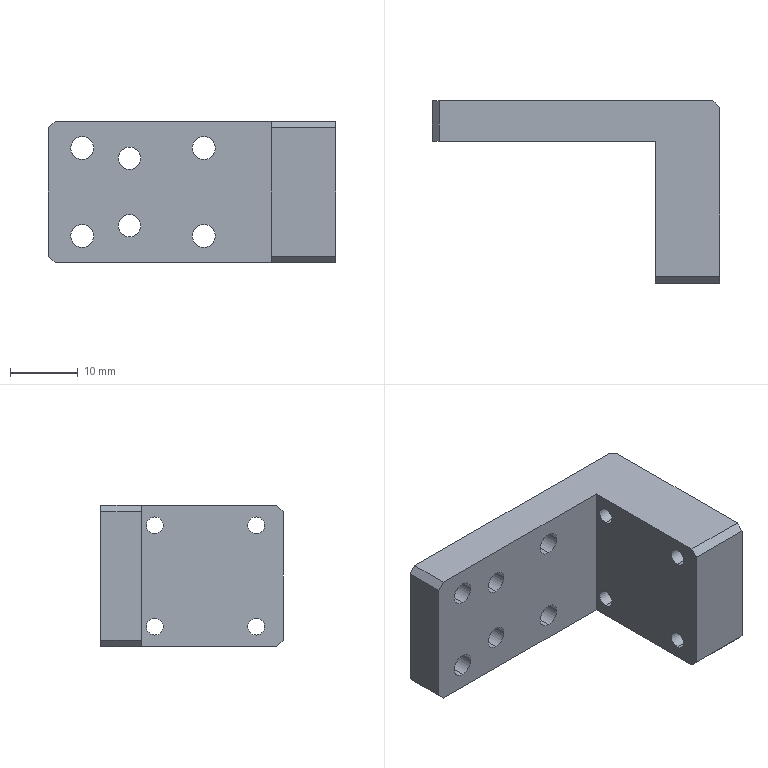Part | STEP file | FBDS-CS-002 | 1 solid | 45 faces | box 42.5 x 27 x 21 mm | volume 8750 mm3 | cylinder 28 | plane 17 | commonest cylinder face diameters 2.5 x8 3.4 x8 6 x8 3.3 x4
STEP:
#1=CARTESIAN_POINT('',(12.,-6.,3.85));
#2=VERTEX_POINT('',#1);
#3=CARTESIAN_POINT('',(12.,-6.,7.15));
#4=VERTEX_POINT('',#3);
#5=CARTESIAN_POINT('',(12.,-6.,5.5));
#6=DIRECTION('',(0.,1.,0.));
#7=DIRECTION('',(-1.,0.,0.));
#8=AXIS2_PLACEMENT_3D('',#5,#6,#7);
#9=CIRCLE('',#8,1.65);
#10=EDGE_CURVE('',#2,#4,#9,.T.);
#11=ORIENTED_EDGE('',*,*,#10,.F.);
#12=CARTESIAN_POINT('',(12.,0.,3.85));
#13=VERTEX_POINT('',#12);
#14=CARTESIAN_POINT('',(12.,0.,3.85));
#15=DIRECTION('',(0.,1.,0.));
#16=VECTOR('',#15,1000.);
#17=LINE('',#14,#16);
#18=EDGE_CURVE('',#2,#13,#17,.T.);
#19=ORIENTED_EDGE('',*,*,#18,.T.);
#20=CARTESIAN_POINT('',(12.,0.,7.15));
#21=VERTEX_POINT('',#20);
#22=CARTESIAN_POINT('',(12.,0.,5.5));
#23=DIRECTION('',(0.,1.,0.));
#24=DIRECTION('',(0.,0.,1.));
#25=AXIS2_PLACEMENT_3D('',#22,#23,#24);
#26=CIRCLE('',#25,1.65);
#27=EDGE_CURVE('',#13,#21,#26,.T.);
#28=ORIENTED_EDGE('',*,*,#27,.T.);
#29=CARTESIAN_POINT('',(12.,0.,7.15));
#30=DIRECTION('',(0.,1.,0.));
#31=VECTOR('',#30,1000.);
#32=LINE('',#29,#31);
#33=EDGE_CURVE('',#4,#21,#32,.T.);
#34=ORIENTED_EDGE('',*,*,#33,.F.);
#35=EDGE_LOOP('',(#11,#19,#28,#34));
#36=FACE_OUTER_BOUND('',#35,.T.);
#37=CARTESIAN_POINT('',(12.,0.,5.5));
#38=DIRECTION('',(0.,1.,0.));
#39=DIRECTION('',(0.,0.,1.));
#40=AXIS2_PLACEMENT_3D('',#37,#38,#39);
#41=CYLINDRICAL_SURFACE('',#40,1.65);
#42=ADVANCED_FACE('',(#36),#41,.F.);
#43=CARTESIAN_POINT('',(12.,-6.,13.85));
#44=VERTEX_POINT('',#43);
#45=CARTESIAN_POINT('',(12.,-6.,17.15));
#46=VERTEX_POINT('',#45);
#47=CARTESIAN_POINT('',(12.,-6.,15.5));
#48=DIRECTION('',(0.,1.,0.));
#49=DIRECTION('',(-1.,0.,0.));
#50=AXIS2_PLACEMENT_3D('',#47,#48,#49);
#51=CIRCLE('',#50,1.65);
#52=EDGE_CURVE('',#44,#46,#51,.T.);
#53=ORIENTED_EDGE('',*,*,#52,.F.);
#54=CARTESIAN_POINT('',(12.,0.,13.85));
#55=VERTEX_POINT('',#54);
#56=CARTESIAN_POINT('',(12.,0.,13.85));
#57=DIRECTION('',(0.,1.,0.));
#58=VECTOR('',#57,1000.);
#59=LINE('',#56,#58);
#60=EDGE_CURVE('',#44,#55,#59,.T.);
#61=ORIENTED_EDGE('',*,*,#60,.T.);
#62=CARTESIAN_POINT('',(12.,0.,17.15));
#63=VERTEX_POINT('',#62);
#64=CARTESIAN_POINT('',(12.,0.,15.5));
#65=DIRECTION('',(0.,1.,0.));
#66=DIRECTION('',(0.,0.,1.));
#67=AXIS2_PLACEMENT_3D('',#64,#65,#66);
#68=CIRCLE('',#67,1.65);
#69=EDGE_CURVE('',#55,#63,#68,.T.);
#70=ORIENTED_EDGE('',*,*,#69,.T.);
#71=CARTESIAN_POINT('',(12.,0.,17.15));
#72=DIRECTION('',(0.,1.,0.));
#73=VECTOR('',#72,1000.);
#74=LINE('',#71,#73);
#75=EDGE_CURVE('',#46,#63,#74,.T.);
#76=ORIENTED_EDGE('',*,*,#75,.F.);
#77=EDGE_LOOP('',(#53,#61,#70,#76));
#78=FACE_OUTER_BOUND('',#77,.T.);
#79=CARTESIAN_POINT('',(12.,0.,15.5));
#80=DIRECTION('',(0.,1.,0.));
#81=DIRECTION('',(0.,0.,1.));
#82=AXIS2_PLACEMENT_3D('',#79,#80,#81);
#83=CYLINDRICAL_SURFACE('',#82,1.65);
#84=ADVANCED_FACE('',(#78),#83,.F.);
#85=CARTESIAN_POINT('',(33.,-8.,4.25));
#86=VERTEX_POINT('',#85);
#87=CARTESIAN_POINT('',(33.,-8.,1.75));
#88=VERTEX_POINT('',#87);
#89=CARTESIAN_POINT('',(33.,-8.,3.));
#90=DIRECTION('',(1.,0.,0.));
#91=DIRECTION('',(0.,0.,-1.));
#92=AXIS2_PLACEMENT_3D('',#89,#90,#91);
#93=CIRCLE('',#92,1.25);
#94=EDGE_CURVE('',#86,#88,#93,.T.);
#95=ORIENTED_EDGE('',*,*,#94,.F.);
#96=CARTESIAN_POINT('',(42.5,-8.,4.25));
#97=VERTEX_POINT('',#96);
#98=CARTESIAN_POINT('',(42.5,-8.,4.25));
#99=DIRECTION('',(1.,0.,0.));
#100=VECTOR('',#99,1000.);
#101=LINE('',#98,#100);
#102=EDGE_CURVE('',#86,#97,#101,.T.);
#103=ORIENTED_EDGE('',*,*,#102,.T.);
#104=CARTESIAN_POINT('',(42.5,-8.,1.75));
#105=VERTEX_POINT('',#104);
#106=CARTESIAN_POINT('',(42.5,-8.,3.));
#107=DIRECTION('',(1.,0.,0.));
#108=DIRECTION('',(0.,0.,-1.));
#109=AXIS2_PLACEMENT_3D('',#106,#107,#108);
#110=CIRCLE('',#109,1.25);
#111=EDGE_CURVE('',#97,#105,#110,.T.);
#112=ORIENTED_EDGE('',*,*,#111,.T.);
#113=CARTESIAN_POINT('',(42.5,-8.,1.75));
#114=DIRECTION('',(1.,0.,0.));
#115=VECTOR('',#114,1000.);
#116=LINE('',#113,#115);
#117=EDGE_CURVE('',#88,#105,#116,.T.);
#118=ORIENTED_EDGE('',*,*,#117,.F.);
#119=EDGE_LOOP('',(#95,#103,#112,#118));
#120=FACE_OUTER_BOUND('',#119,.T.);
#121=CARTESIAN_POINT('',(42.5,-8.,3.));
#122=DIRECTION('',(1.,0.,0.));
#123=DIRECTION('',(0.,0.,-1.));
#124=AXIS2_PLACEMENT_3D('',#121,#122,#123);
#125=CYLINDRICAL_SURFACE('',#124,1.25);
#126=ADVANCED_FACE('',(#120),#125,.F.);
#127=CARTESIAN_POINT('',(33.,-8.,19.25));
#128=VERTEX_POINT('',#127);
#129=CARTESIAN_POINT('',(33.,-8.,16.75));
#130=VERTEX_POINT('',#129);
#131=CARTESIAN_POINT('',(33.,-8.,18.));
#132=DIRECTION('',(1.,0.,0.));
#133=DIRECTION('',(0.,0.,-1.));
#134=AXIS2_PLACEMENT_3D('',#131,#132,#133);
#135=CIRCLE('',#134,1.25);
#136=EDGE_CURVE('',#128,#130,#135,.T.);
#137=ORIENTED_EDGE('',*,*,#136,.F.);
#138=CARTESIAN_POINT('',(42.5,-8.,19.25));
#139=VERTEX_POINT('',#138);
#140=CARTESIAN_POINT('',(42.5,-8.,19.25));
#141=DIRECTION('',(1.,0.,0.));
#142=VECTOR('',#141,1000.);
#143=LINE('',#140,#142);
#144=EDGE_CURVE('',#128,#139,#143,.T.);
#145=ORIENTED_EDGE('',*,*,#144,.T.);
#146=CARTESIAN_POINT('',(42.5,-8.,16.75));
#147=VERTEX_POINT('',#146);
#148=CARTESIAN_POINT('',(42.5,-8.,18.));
#149=DIRECTION('',(1.,0.,0.));
#150=DIRECTION('',(0.,0.,-1.));
#151=AXIS2_PLACEMENT_3D('',#148,#149,#150);
#152=CIRCLE('',#151,1.25);
#153=EDGE_CURVE('',#139,#147,#152,.T.);
#154=ORIENTED_EDGE('',*,*,#153,.T.);
#155=CARTESIAN_POINT('',(42.5,-8.,16.75));
#156=DIRECTION('',(1.,0.,0.));
#157=VECTOR('',#156,1000.);
#158=LINE('',#155,#157);
#159=EDGE_CURVE('',#130,#147,#158,.T.);
#160=ORIENTED_EDGE('',*,*,#159,.F.);
#161=EDGE_LOOP('',(#137,#145,#154,#160));
#162=FACE_OUTER_BOUND('',#161,.T.);
#163=CARTESIAN_POINT('',(42.5,-8.,18.));
#164=DIRECTION('',(1.,0.,0.));
#165=DIRECTION('',(0.,0.,-1.));
#166=AXIS2_PLACEMENT_3D('',#163,#164,#165);
#167=CYLINDRICAL_SURFACE('',#166,1.25);
#168=ADVANCED_FACE('',(#162),#167,.F.);
#169=CARTESIAN_POINT('',(33.,-23.,4.25));
#170=VERTEX_POINT('',#169);
#171=CARTESIAN_POINT('',(33.,-23.,1.75));
#172=VERTEX_POINT('',#171);
#173=CARTESIAN_POINT('',(33.,-23.,3.));
#174=DIRECTION('',(1.,0.,0.));
#175=DIRECTION('',(0.,0.,-1.));
#176=AXIS2_PLACEMENT_3D('',#173,#174,#175);
#177=CIRCLE('',#176,1.25);
#178=EDGE_CURVE('',#170,#172,#177,.T.);
#179=ORIENTED_EDGE('',*,*,#178,.F.);
#180=CARTESIAN_POINT('',(42.5,-23.,4.25));
#181=VERTEX_POINT('',#180);
#182=CARTESIAN_POINT('',(42.5,-23.,4.25));
#183=DIRECTION('',(1.,0.,0.));
#184=VECTOR('',#183,1000.);
#185=LINE('',#182,#184);
#186=EDGE_CURVE('',#170,#181,#185,.T.);
#187=ORIENTED_EDGE('',*,*,#186,.T.);
#188=CARTESIAN_POINT('',(42.5,-23.,1.75));
#189=VERTEX_POINT('',#188);
#190=CARTESIAN_POINT('',(42.5,-23.,3.));
#191=DIRECTION('',(1.,0.,0.));
#192=DIRECTION('',(0.,0.,-1.));
#193=AXIS2_PLACEMENT_3D('',#190,#191,#192);
#194=CIRCLE('',#193,1.25);
#195=EDGE_CURVE('',#181,#189,#194,.T.);
#196=ORIENTED_EDGE('',*,*,#195,.T.);
#197=CARTESIAN_POINT('',(42.5,-23.,1.75));
#198=DIRECTION('',(1.,0.,0.));
#199=VECTOR('',#198,1000.);
#200=LINE('',#197,#199);
#201=EDGE_CURVE('',#172,#189,#200,.T.);
#202=ORIENTED_EDGE('',*,*,#201,.F.);
#203=EDGE_LOOP('',(#179,#187,#196,#202));
#204=FACE_OUTER_BOUND('',#203,.T.);
#205=CARTESIAN_POINT('',(42.5,-23.,3.));
#206=DIRECTION('',(1.,0.,0.));
#207=DIRECTION('',(0.,0.,-1.));
#208=AXIS2_PLACEMENT_3D('',#205,#206,#207);
#209=CYLINDRICAL_SURFACE('',#208,1.25);
#210=ADVANCED_FACE('',(#204),#209,.F.);
#211=CARTESIAN_POINT('',(33.,-23.,19.25));
#212=VERTEX_POINT('',#211);
#213=CARTESIAN_POINT('',(33.,-23.,16.75));
#214=VERTEX_POINT('',#213);
#215=CARTESIAN_POINT('',(33.,-23.,18.));
#216=DIRECTION('',(1.,0.,0.));
#217=DIRECTION('',(0.,0.,-1.));
#218=AXIS2_PLACEMENT_3D('',#215,#216,#217);
#219=CIRCLE('',#218,1.25);
#220=EDGE_CURVE('',#212,#214,#219,.T.);
#221=ORIENTED_EDGE('',*,*,#220,.F.);
#222=CARTESIAN_POINT('',(42.5,-23.,19.25));
#223=VERTEX_POINT('',#222);
#224=CARTESIAN_POINT('',(42.5,-23.,19.25));
#225=DIRECTION('',(1.,0.,0.));
#226=VECTOR('',#225,1000.);
#227=LINE('',#224,#226);
#228=EDGE_CURVE('',#212,#223,#227,.T.);
#229=ORIENTED_EDGE('',*,*,#228,.T.);
#230=CARTESIAN_POINT('',(42.5,-23.,16.75));
#231=VERTEX_POINT('',#230);
#232=CARTESIAN_POINT('',(42.5,-23.,18.));
#233=DIRECTION('',(1.,0.,0.));
#234=DIRECTION('',(0.,0.,-1.));
#235=AXIS2_PLACEMENT_3D('',#232,#233,#234);
#236=CIRCLE('',#235,1.25);
#237=EDGE_CURVE('',#223,#231,#236,.T.);
#238=ORIENTED_EDGE('',*,*,#237,.T.);
#239=CARTESIAN_POINT('',(42.5,-23.,16.75));
#240=DIRECTION('',(1.,0.,0.));
#241=VECTOR('',#240,1000.);
#242=LINE('',#239,#241);
#243=EDGE_CURVE('',#214,#231,#242,.T.);
#244=ORIENTED_EDGE('',*,*,#243,.F.);
#245=EDGE_LOOP('',(#221,#229,#238,#244));
#246=FACE_OUTER_BOUND('',#245,.T.);
#247=CARTESIAN_POINT('',(42.5,-23.,18.));
#248=DIRECTION('',(1.,0.,0.));
#249=DIRECTION('',(0.,0.,-1.));
#250=AXIS2_PLACEMENT_3D('',#247,#248,#249);
#251=CYLINDRICAL_SURFACE('',#250,1.25);
#252=ADVANCED_FACE('',(#246),#251,.F.);
#253=CARTESIAN_POINT('',(5.,-3.4,1.));
#254=VERTEX_POINT('',#253);
#255=CARTESIAN_POINT('',(5.,-3.4,7.));
#256=VERTEX_POINT('',#255);
#257=CARTESIAN_POINT('',(5.,-3.4,4.));
#258=DIRECTION('',(0.,1.,0.));
#259=DIRECTION('',(0.,0.,1.));
#260=AXIS2_PLACEMENT_3D('',#257,#258,#259);
#261=CIRCLE('',#260,3.);
#262=EDGE_CURVE('',#254,#256,#261,.T.);
#263=ORIENTED_EDGE('',*,*,#262,.F.);
#264=CARTESIAN_POINT('',(5.,0.,1.));
#265=VERTEX_POINT('',#264);
#266=CARTESIAN_POINT('',(5.,0.,1.));
#267=DIRECTION('',(0.,1.,0.));
#268=VECTOR('',#267,1000.);
#269=LINE('',#266,#268);
#270=EDGE_CURVE('',#254,#265,#269,.T.);
#271=ORIENTED_EDGE('',*,*,#270,.T.);
#272=CARTESIAN_POINT('',(5.,0.,7.));
#273=VERTEX_POINT('',#272);
#274=CARTESIAN_POINT('',(5.,0.,4.));
#275=DIRECTION('',(0.,1.,0.));
#276=DIRECTION('',(0.,0.,1.));
#277=AXIS2_PLACEMENT_3D('',#274,#275,#276);
#278=CIRCLE('',#277,3.);
#279=EDGE_CURVE('',#265,#273,#278,.T.);
#280=ORIENTED_EDGE('',*,*,#279,.T.);
#281=CARTESIAN_POINT('',(5.,0.,7.));
#282=DIRECTION('',(0.,1.,0.));
#283=VECTOR('',#282,1000.);
#284=LINE('',#281,#283);
#285=EDGE_CURVE('',#256,#273,#284,.T.);
#286=ORIENTED_EDGE('',*,*,#285,.F.);
#287=EDGE_LOOP('',(#263,#271,#280,#286));
#288=FACE_OUTER_BOUND('',#287,.T.);
#289=CARTESIAN_POINT('',(5.,0.,4.));
#290=DIRECTION('',(0.,1.,0.));
#291=DIRECTION('',(0.,0.,1.));
#292=AXIS2_PLACEMENT_3D('',#289,#290,#291);
#293=CYLINDRICAL_SURFACE('',#292,3.);
#294=ADVANCED_FACE('',(#288),#293,.F.);
#295=CARTESIAN_POINT('',(5.,-6.,2.3));
#296=VERTEX_POINT('',#295);
#297=CARTESIAN_POINT('',(5.,-6.,5.7));
#298=VERTEX_POINT('',#297);
#299=CARTESIAN_POINT('',(5.,-6.,4.));
#300=DIRECTION('',(0.,1.,0.));
#301=DIRECTION('',(-1.,0.,0.));
#302=AXIS2_PLACEMENT_3D('',#299,#300,#301);
#303=CIRCLE('',#302,1.7);
#304=EDGE_CURVE('',#296,#298,#303,.T.);
#305=ORIENTED_EDGE('',*,*,#304,.F.);
#306=CARTESIAN_POINT('',(5.,-3.4,2.3));
#307=VERTEX_POINT('',#306);
#308=CARTESIAN_POINT('',(5.,0.,2.3));
#309=DIRECTION('',(0.,1.,0.));
#310=VECTOR('',#309,1000.);
#311=LINE('',#308,#310);
#312=EDGE_CURVE('',#296,#307,#311,.T.);
#313=ORIENTED_EDGE('',*,*,#312,.T.);
#314=CARTESIAN_POINT('',(5.,-3.4,5.7));
#315=VERTEX_POINT('',#314);
#316=CARTESIAN_POINT('',(5.,-3.4,4.));
#317=DIRECTION('',(0.,1.,0.));
#318=DIRECTION('',(0.,0.,1.));
#319=AXIS2_PLACEMENT_3D('',#316,#317,#318);
#320=CIRCLE('',#319,1.7);
#321=EDGE_CURVE('',#307,#315,#320,.T.);
#322=ORIENTED_EDGE('',*,*,#321,.T.);
#323=CARTESIAN_POINT('',(5.,0.,5.7));
#324=DIRECTION('',(0.,1.,0.));
#325=VECTOR('',#324,1000.);
#326=LINE('',#323,#325);
#327=EDGE_CURVE('',#298,#315,#326,.T.);
#328=ORIENTED_EDGE('',*,*,#327,.F.);
#329=EDGE_LOOP('',(#305,#313,#322,#328));
#330=FACE_OUTER_BOUND('',#329,.T.);
#331=CARTESIAN_POINT('',(5.,0.,4.));
#332=DIRECTION('',(0.,1.,0.));
#333=DIRECTION('',(0.,0.,1.));
#334=AXIS2_PLACEMENT_3D('',#331,#332,#333);
#335=CYLINDRICAL_SURFACE('',#334,1.7);
#336=ADVANCED_FACE('',(#330),#335,.F.);
#337=CARTESIAN_POINT('',(23.,-3.4,1.));
#338=VERTEX_POINT('',#337);
#339=CARTESIAN_POINT('',(23.,-3.4,7.));
#340=VERTEX_POINT('',#339);
#341=CARTESIAN_POINT('',(23.,-3.4,4.));
#342=DIRECTION('',(0.,1.,0.));
#343=DIRECTION('',(0.,0.,1.));
#344=AXIS2_PLACEMENT_3D('',#341,#342,#343);
#345=CIRCLE('',#344,3.);
#346=EDGE_CURVE('',#338,#340,#345,.T.);
#347=ORIENTED_EDGE('',*,*,#346,.F.);
#348=CARTESIAN_POINT('',(23.,0.,1.));
#349=VERTEX_POINT('',#348);
#350=CARTESIAN_POINT('',(23.,0.,1.));
#351=DIRECTION('',(0.,1.,0.));
#352=VECTOR('',#351,1000.);
#353=LINE('',#350,#352);
#354=EDGE_CURVE('',#338,#349,#353,.T.);
#355=ORIENTED_EDGE('',*,*,#354,.T.);
#356=CARTESIAN_POINT('',(23.,0.,7.));
#357=VERTEX_POINT('',#356);
#358=CARTESIAN_POINT('',(23.,0.,4.));
#359=DIRECTION('',(0.,1.,0.));
#360=DIRECTION('',(0.,0.,1.));
#361=AXIS2_PLACEMENT_3D('',#358,#359,#360);
#362=CIRCLE('',#361,3.);
#363=EDGE_CURVE('',#349,#357,#362,.T.);
#364=ORIENTED_EDGE('',*,*,#363,.T.);
#365=CARTESIAN_POINT('',(23.,0.,7.));
#366=DIRECTION('',(0.,1.,0.));
#367=VECTOR('',#366,1000.);
#368=LINE('',#365,#367);
#369=EDGE_CURVE('',#340,#357,#368,.T.);
#370=ORIENTED_EDGE('',*,*,#369,.F.);
#371=EDGE_LOOP('',(#347,#355,#364,#370));
#372=FACE_OUTER_BOUND('',#371,.T.);
#373=CARTESIAN_POINT('',(23.,0.,4.));
#374=DIRECTION('',(0.,1.,0.));
#375=DIRECTION('',(0.,0.,1.));
#376=AXIS2_PLACEMENT_3D('',#373,#374,#375);
#377=CYLINDRICAL_SURFACE('',#376,3.);
#378=ADVANCED_FACE('',(#372),#377,.F.);
#379=CARTESIAN_POINT('',(23.,-6.,2.3));
#380=VERTEX_POINT('',#379);
#381=CARTESIAN_POINT('',(23.,-6.,5.7));
#382=VERTEX_POINT('',#381);
#383=CARTESIAN_POINT('',(23.,-6.,4.));
#384=DIRECTION('',(0.,1.,0.));
#385=DIRECTION('',(-1.,0.,0.));
#386=AXIS2_PLACEMENT_3D('',#383,#384,#385);
#387=CIRCLE('',#386,1.7);
#388=EDGE_CURVE('',#380,#382,#387,.T.);
#389=ORIENTED_EDGE('',*,*,#388,.F.);
#390=CARTESIAN_POINT('',(23.,-3.4,2.3));
#391=VERTEX_POINT('',#390);
#392=CARTESIAN_POINT('',(23.,0.,2.3));
#393=DIRECTION('',(0.,1.,0.));
#394=VECTOR('',#393,1000.);
#395=LINE('',#392,#394);
#396=EDGE_CURVE('',#380,#391,#395,.T.);
#397=ORIENTED_EDGE('',*,*,#396,.T.);
#398=CARTESIAN_POINT('',(23.,-3.4,5.7));
#399=VERTEX_POINT('',#398);
#400=CARTESIAN_POINT('',(23.,-3.4,4.));
#401=DIRECTION('',(0.,1.,0.));
#402=DIRECTION('',(0.,0.,1.));
#403=AXIS2_PLACEMENT_3D('',#400,#401,#402);
#404=CIRCLE('',#403,1.7);
#405=EDGE_CURVE('',#391,#399,#404,.T.);
#406=ORIENTED_EDGE('',*,*,#405,.T.);
#407=CARTESIAN_POINT('',(23.,0.,5.7));
#408=DIRECTION('',(0.,1.,0.));
#409=VECTOR('',#408,1000.);
#410=LINE('',#407,#409);
#411=EDGE_CURVE('',#382,#399,#410,.T.);
#412=ORIENTED_EDGE('',*,*,#411,.F.);
#413=EDGE_LOOP('',(#389,#397,#406,#412));
#414=FACE_OUTER_BOUND('',#413,.T.);
#415=CARTESIAN_POINT('',(23.,0.,4.));
#416=DIRECTION('',(0.,1.,0.));
#417=DIRECTION('',(0.,0.,1.));
#418=AXIS2_PLACEMENT_3D('',#415,#416,#417);
#419=CYLINDRICAL_SURFACE('',#418,1.7);
#420=ADVANCED_FACE('',(#414),#419,.F.);
#421=CARTESIAN_POINT('',(23.,-3.4,14.));
#422=VERTEX_POINT('',#421);
#423=CARTESIAN_POINT('',(23.,-3.4,20.));
#424=VERTEX_POINT('',#423);
#425=CARTESIAN_POINT('',(23.,-3.4,17.));
#426=DIRECTION('',(0.,1.,0.));
#427=DIRECTION('',(0.,0.,1.));
#428=AXIS2_PLACEMENT_3D('',#425,#426,#427);
#429=CIRCLE('',#428,3.);
#430=EDGE_CURVE('',#422,#424,#429,.T.);
#431=ORIENTED_EDGE('',*,*,#430,.F.);
#432=CARTESIAN_POINT('',(23.,0.,14.));
#433=VERTEX_POINT('',#432);
#434=CARTESIAN_POINT('',(23.,0.,14.));
#435=DIRECTION('',(0.,1.,0.));
#436=VECTOR('',#435,1000.);
#437=LINE('',#434,#436);
#438=EDGE_CURVE('',#422,#433,#437,.T.);
#439=ORIENTED_EDGE('',*,*,#438,.T.);
#440=CARTESIAN_POINT('',(23.,0.,20.));
#441=VERTEX_POINT('',#440);
#442=CARTESIAN_POINT('',(23.,0.,17.));
#443=DIRECTION('',(0.,1.,0.));
#444=DIRECTION('',(0.,0.,1.));
#445=AXIS2_PLACEMENT_3D('',#442,#443,#444);
#446=CIRCLE('',#445,3.);
#447=EDGE_CURVE('',#433,#441,#446,.T.);
#448=ORIENTED_EDGE('',*,*,#447,.T.);
#449=CARTESIAN_POINT('',(23.,0.,20.));
#450=DIRECTION('',(0.,1.,0.));
#451=VECTOR('',#450,1000.);
#452=LINE('',#449,#451);
#453=EDGE_CURVE('',#424,#441,#452,.T.);
#454=ORIENTED_EDGE('',*,*,#453,.F.);
#455=EDGE_LOOP('',(#431,#439,#448,#454));
#456=FACE_OUTER_BOUND('',#455,.T.);
#457=CARTESIAN_POINT('',(23.,0.,17.));
#458=DIRECTION('',(0.,1.,0.));
#459=DIRECTION('',(0.,0.,1.));
#460=AXIS2_PLACEMENT_3D('',#457,#458,#459);
#461=CYLINDRICAL_SURFACE('',#460,3.);
#462=ADVANCED_FACE('',(#456),#461,.F.);
#463=CARTESIAN_POINT('',(23.,-6.,15.3));
#464=VERTEX_POINT('',#463);
#465=CARTESIAN_POINT('',(23.,-6.,18.7));
#466=VERTEX_POINT('',#465);
#467=CARTESIAN_POINT('',(23.,-6.,17.));
#468=DIRECTION('',(0.,1.,0.));
#469=DIRECTION('',(-1.,0.,0.));
#470=AXIS2_PLACEMENT_3D('',#467,#468,#469);
#471=CIRCLE('',#470,1.7);
#472=EDGE_CURVE('',#464,#466,#471,.T.);
#473=ORIENTED_EDGE('',*,*,#472,.F.);
#474=CARTESIAN_POINT('',(23.,-3.4,15.3));
#475=VERTEX_POINT('',#474);
#476=CARTESIAN_POINT('',(23.,0.,15.3));
#477=DIRECTION('',(0.,1.,0.));
#478=VECTOR('',#477,1000.);
#479=LINE('',#476,#478);
#480=EDGE_CURVE('',#464,#475,#479,.T.);
#481=ORIENTED_EDGE('',*,*,#480,.T.);
#482=CARTESIAN_POINT('',(23.,-3.4,18.7));
#483=VERTEX_POINT('',#482);
#484=CARTESIAN_POINT('',(23.,-3.4,17.));
#485=DIRECTION('',(0.,1.,0.));
#486=DIRECTION('',(0.,0.,1.));
#487=AXIS2_PLACEMENT_3D('',#484,#485,#486);
#488=CIRCLE('',#487,1.7);
#489=EDGE_CURVE('',#475,#483,#488,.T.);
#490=ORIENTED_EDGE('',*,*,#489,.T.);
#491=CARTESIAN_POINT('',(23.,0.,18.7));
#492=DIRECTION('',(0.,1.,0.));
#493=VECTOR('',#492,1000.);
#494=LINE('',#491,#493);
#495=EDGE_CURVE('',#466,#483,#494,.T.);
#496=ORIENTED_EDGE('',*,*,#495,.F.);
#497=EDGE_LOOP('',(#473,#481,#490,#496));
#498=FACE_OUTER_BOUND('',#497,.T.);
#499=CARTESIAN_POINT('',(23.,0.,17.));
#500=DIRECTION('',(0.,1.,0.));
#501=DIRECTION('',(0.,0.,1.));
#502=AXIS2_PLACEMENT_3D('',#499,#500,#501);
#503=CYLINDRICAL_SURFACE('',#502,1.7);
#504=ADVANCED_FACE('',(#498),#503,.F.);
#505=CARTESIAN_POINT('',(5.,-3.4,14.));
#506=VERTEX_POINT('',#505);
#507=CARTESIAN_POINT('',(5.,-3.4,20.));
#508=VERTEX_POINT('',#507);
#509=CARTESIAN_POINT('',(5.,-3.4,17.));
#510=DIRECTION('',(0.,1.,0.));
#511=DIRECTION('',(0.,0.,1.));
#512=AXIS2_PLACEMENT_3D('',#509,#510,#511);
#513=CIRCLE('',#512,3.);
#514=EDGE_CURVE('',#506,#508,#513,.T.);
#515=ORIENTED_EDGE('',*,*,#514,.F.);
#516=CARTESIAN_POINT('',(5.,0.,14.));
#517=VERTEX_POINT('',#516);
#518=CARTESIAN_POINT('',(5.,0.,14.));
#519=DIRECTION('',(0.,1.,0.));
#520=VECTOR('',#519,1000.);
#521=LINE('',#518,#520);
#522=EDGE_CURVE('',#506,#517,#521,.T.);
#523=ORIENTED_EDGE('',*,*,#522,.T.);
#524=CARTESIAN_POINT('',(5.,0.,20.));
#525=VERTEX_POINT('',#524);
#526=CARTESIAN_POINT('',(5.,0.,17.));
#527=DIRECTION('',(0.,1.,0.));
#528=DIRECTION('',(0.,0.,1.));
#529=AXIS2_PLACEMENT_3D('',#526,#527,#528);
#530=CIRCLE('',#529,3.);
#531=EDGE_CURVE('',#517,#525,#530,.T.);
#532=ORIENTED_EDGE('',*,*,#531,.T.);
#533=CARTESIAN_POINT('',(5.,0.,20.));
#534=DIRECTION('',(0.,1.,0.));
#535=VECTOR('',#534,1000.);
#536=LINE('',#533,#535);
#537=EDGE_CURVE('',#508,#525,#536,.T.);
#538=ORIENTED_EDGE('',*,*,#537,.F.);
#539=EDGE_LOOP('',(#515,#523,#532,#538));
#540=FACE_OUTER_BOUND('',#539,.T.);
#541=CARTESIAN_POINT('',(5.,0.,17.));
#542=DIRECTION('',(0.,1.,0.));
#543=DIRECTION('',(0.,0.,1.));
#544=AXIS2_PLACEMENT_3D('',#541,#542,#543);
#545=CYLINDRICAL_SURFACE('',#544,3.);
#546=ADVANCED_FACE('',(#540),#545,.F.);
#547=CARTESIAN_POINT('',(5.,-6.,15.3));
#548=VERTEX_POINT('',#547);
#549=CARTESIAN_POINT('',(5.,-6.,18.7));
#550=VERTEX_POINT('',#549);
#551=CARTESIAN_POINT('',(5.,-6.,17.));
#552=DIRECTION('',(0.,1.,0.));
#553=DIRECTION('',(-1.,0.,0.));
#554=AXIS2_PLACEMENT_3D('',#551,#552,#553);
#555=CIRCLE('',#554,1.7);
#556=EDGE_CURVE('',#548,#550,#555,.T.);
#557=ORIENTED_EDGE('',*,*,#556,.F.);
#558=CARTESIAN_POINT('',(5.,-3.4,15.3));
#559=VERTEX_POINT('',#558);
#560=CARTESIAN_POINT('',(5.,0.,15.3));
#561=DIRECTION('',(0.,1.,0.));
#562=VECTOR('',#561,1000.);
#563=LINE('',#560,#562);
#564=EDGE_CURVE('',#548,#559,#563,.T.);
#565=ORIENTED_EDGE('',*,*,#564,.T.);
#566=CARTESIAN_POINT('',(5.,-3.4,18.7));
#567=VERTEX_POINT('',#566);
#568=CARTESIAN_POINT('',(5.,-3.4,17.));
#569=DIRECTION('',(0.,1.,0.));
#570=DIRECTION('',(0.,0.,1.));
#571=AXIS2_PLACEMENT_3D('',#568,#569,#570);
#572=CIRCLE('',#571,1.7);
#573=EDGE_CURVE('',#559,#567,#572,.T.);
#574=ORIENTED_EDGE('',*,*,#573,.T.);
#575=CARTESIAN_POINT('',(5.,0.,18.7));
#576=DIRECTION('',(0.,1.,0.));
#577=VECTOR('',#576,1000.);
#578=LINE('',#575,#577);
#579=EDGE_CURVE('',#550,#567,#578,.T.);
#580=ORIENTED_EDGE('',*,*,#579,.F.);
#581=EDGE_LOOP('',(#557,#565,#574,#580));
#582=FACE_OUTER_BOUND('',#581,.T.);
#583=CARTESIAN_POINT('',(5.,0.,17.));
#584=DIRECTION('',(0.,1.,0.));
#585=DIRECTION('',(0.,0.,1.));
#586=AXIS2_PLACEMENT_3D('',#583,#584,#585);
#587=CYLINDRICAL_SURFACE('',#586,1.7);
#588=ADVANCED_FACE('',(#582),#587,.F.);
#589=CARTESIAN_POINT('',(0.,-6.,20.));
#590=VERTEX_POINT('',#589);
#591=CARTESIAN_POINT('',(0.,-6.,1.));
#592=VERTEX_POINT('',#591);
#593=CARTESIAN_POINT('',(0.,-6.,21.));
#594=DIRECTION('',(0.,0.,-1.));
#595=VECTOR('',#594,1000.);
#596=LINE('',#593,#595);
#597=EDGE_CURVE('',#590,#592,#596,.T.);
#598=ORIENTED_EDGE('',*,*,#597,.F.);
#599=CARTESIAN_POINT('',(0.,0.,20.));
#600=VERTEX_POINT('',#599);
#601=CARTESIAN_POINT('',(0.,-6.,20.));
#602=DIRECTION('',(0.,1.,0.));
#603=VECTOR('',#602,1000.);
#604=LINE('',#601,#603);
#605=EDGE_CURVE('',#590,#600,#604,.T.);
#606=ORIENTED_EDGE('',*,*,#605,.T.);
#607=CARTESIAN_POINT('',(0.,0.,1.));
#608=VERTEX_POINT('',#607);
#609=CARTESIAN_POINT('',(0.,0.,21.));
#610=DIRECTION('',(0.,0.,-1.));
#611=VECTOR('',#610,1000.);
#612=LINE('',#609,#611);
#613=EDGE_CURVE('',#600,#608,#612,.T.);
#614=ORIENTED_EDGE('',*,*,#613,.T.);
#615=CARTESIAN_POINT('',(0.,-6.,1.));
#616=DIRECTION('',(0.,-1.,0.));
#617=VECTOR('',#616,1000.);
#618=LINE('',#615,#617);
#619=EDGE_CURVE('',#608,#592,#618,.T.);
#620=ORIENTED_EDGE('',*,*,#619,.T.);
#621=EDGE_LOOP('',(#598,#606,#614,#620));
#622=FACE_OUTER_BOUND('',#621,.T.);
#623=CARTESIAN_POINT('',(0.,-6.,21.));
#624=DIRECTION('',(1.,0.,0.));
#625=DIRECTION('',(0.,0.,-1.));
#626=AXIS2_PLACEMENT_3D('',#623,#624,#625);
#627=PLANE('',#626);
#628=ADVANCED_FACE('',(#622),#627,.F.);
#629=CARTESIAN_POINT('',(12.,-6.,5.5));
#630=DIRECTION('',(0.,1.,0.));
#631=DIRECTION('',(-1.,0.,0.));
#632=AXIS2_PLACEMENT_3D('',#629,#630,#631);
#633=CIRCLE('',#632,1.65);
#634=EDGE_CURVE('',#4,#2,#633,.T.);
#635=ORIENTED_EDGE('',*,*,#634,.T.);
#636=ORIENTED_EDGE('',*,*,#10,.T.);
#637=EDGE_LOOP('',(#635,#636));
#638=FACE_BOUND('',#637,.T.);
#639=CARTESIAN_POINT('',(12.,-6.,15.5));
#640=DIRECTION('',(0.,1.,0.));
#641=DIRECTION('',(-1.,0.,0.));
#642=AXIS2_PLACEMENT_3D('',#639,#640,#641);
#643=CIRCLE('',#642,1.65);
#644=EDGE_CURVE('',#46,#44,#643,.T.);
#645=ORIENTED_EDGE('',*,*,#644,.T.);
#646=ORIENTED_EDGE('',*,*,#52,.T.);
#647=EDGE_LOOP('',(#645,#646));
#648=FACE_BOUND('',#647,.T.);
#649=CARTESIAN_POINT('',(5.,-6.,4.));
#650=DIRECTION('',(0.,1.,0.));
#651=DIRECTION('',(-1.,0.,0.));
#652=AXIS2_PLACEMENT_3D('',#649,#650,#651);
#653=CIRCLE('',#652,1.7);
#654=EDGE_CURVE('',#298,#296,#653,.T.);
#655=ORIENTED_EDGE('',*,*,#654,.T.);
#656=ORIENTED_EDGE('',*,*,#304,.T.);
#657=EDGE_LOOP('',(#655,#656));
#658=FACE_BOUND('',#657,.T.);
#659=CARTESIAN_POINT('',(23.,-6.,4.));
#660=DIRECTION('',(0.,1.,0.));
#661=DIRECTION('',(-1.,0.,0.));
#662=AXIS2_PLACEMENT_3D('',#659,#660,#661);
#663=CIRCLE('',#662,1.7);
#664=EDGE_CURVE('',#382,#380,#663,.T.);
#665=ORIENTED_EDGE('',*,*,#664,.T.);
#666=ORIENTED_EDGE('',*,*,#388,.T.);
#667=EDGE_LOOP('',(#665,#666));
#668=FACE_BOUND('',#667,.T.);
#669=CARTESIAN_POINT('',(23.,-6.,17.));
#670=DIRECTION('',(0.,1.,0.));
#671=DIRECTION('',(-1.,0.,0.));
#672=AXIS2_PLACEMENT_3D('',#669,#670,#671);
#673=CIRCLE('',#672,1.7);
#674=EDGE_CURVE('',#466,#464,#673,.T.);
#675=ORIENTED_EDGE('',*,*,#674,.T.);
#676=ORIENTED_EDGE('',*,*,#472,.T.);
#677=EDGE_LOOP('',(#675,#676));
#678=FACE_BOUND('',#677,.T.);
#679=CARTESIAN_POINT('',(5.,-6.,17.));
#680=DIRECTION('',(0.,1.,0.));
#681=DIRECTION('',(-1.,0.,0.));
#682=AXIS2_PLACEMENT_3D('',#679,#680,#681);
#683=CIRCLE('',#682,1.7);
#684=EDGE_CURVE('',#550,#548,#683,.T.);
#685=ORIENTED_EDGE('',*,*,#684,.T.);
#686=ORIENTED_EDGE('',*,*,#556,.T.);
#687=EDGE_LOOP('',(#685,#686));
#688=FACE_BOUND('',#687,.T.);
#689=CARTESIAN_POINT('',(1.,-6.,21.));
#690=VERTEX_POINT('',#689);
#691=CARTESIAN_POINT('',(33.,-6.,21.));
#692=VERTEX_POINT('',#691);
#693=CARTESIAN_POINT('',(33.,-6.,21.));
#694=DIRECTION('',(1.,0.,0.));
#695=VECTOR('',#694,1000.);
#696=LINE('',#693,#695);
#697=EDGE_CURVE('',#690,#692,#696,.T.);
#698=ORIENTED_EDGE('',*,*,#697,.F.);
#699=CARTESIAN_POINT('',(1.,-6.,21.));
#700=DIRECTION('',(-0.7071,0.,-0.7071));
#701=VECTOR('',#700,1000.);
#702=LINE('',#699,#701);
#703=EDGE_CURVE('',#690,#590,#702,.T.);
#704=ORIENTED_EDGE('',*,*,#703,.T.);
#705=ORIENTED_EDGE('',*,*,#597,.T.);
#706=CARTESIAN_POINT('',(1.,-6.,0.));
#707=VERTEX_POINT('',#706);
#708=CARTESIAN_POINT('',(0.,-6.,1.));
#709=DIRECTION('',(0.7071,0.,-0.7071));
#710=VECTOR('',#709,1000.);
#711=LINE('',#708,#710);
#712=EDGE_CURVE('',#592,#707,#711,.T.);
#713=ORIENTED_EDGE('',*,*,#712,.T.);
#714=CARTESIAN_POINT('',(33.,-6.,0.));
#715=VERTEX_POINT('',#714);
#716=CARTESIAN_POINT('',(33.,-6.,0.));
#717=DIRECTION('',(1.,0.,0.));
#718=VECTOR('',#717,1000.);
#719=LINE('',#716,#718);
#720=EDGE_CURVE('',#707,#715,#719,.T.);
#721=ORIENTED_EDGE('',*,*,#720,.T.);
#722=CARTESIAN_POINT('',(33.,-6.,21.));
#723=DIRECTION('',(0.,0.,-1.));
#724=VECTOR('',#723,1000.);
#725=LINE('',#722,#724);
#726=EDGE_CURVE('',#692,#715,#725,.T.);
#727=ORIENTED_EDGE('',*,*,#726,.F.);
#728=EDGE_LOOP('',(#698,#704,#705,#713,#721,#727));
#729=FACE_OUTER_BOUND('',#728,.T.);
#730=CARTESIAN_POINT('',(33.,-6.,21.));
#731=DIRECTION('',(0.,1.,0.));
#732=DIRECTION('',(-1.,0.,0.));
#733=AXIS2_PLACEMENT_3D('',#730,#731,#732);
#734=PLANE('',#733);
#735=ADVANCED_FACE('',(#638,#648,#658,#668,#678,#688,#729),#734,.F.);
#736=CARTESIAN_POINT('',(33.,-8.,3.));
#737=DIRECTION('',(1.,0.,0.));
#738=DIRECTION('',(0.,0.,-1.));
#739=AXIS2_PLACEMENT_3D('',#736,#737,#738);
#740=CIRCLE('',#739,1.25);
#741=EDGE_CURVE('',#88,#86,#740,.T.);
#742=ORIENTED_EDGE('',*,*,#741,.T.);
#743=ORIENTED_EDGE('',*,*,#94,.T.);
#744=EDGE_LOOP('',(#742,#743));
#745=FACE_BOUND('',#744,.T.);
#746=CARTESIAN_POINT('',(33.,-8.,18.));
#747=DIRECTION('',(1.,0.,0.));
#748=DIRECTION('',(0.,0.,-1.));
#749=AXIS2_PLACEMENT_3D('',#746,#747,#748);
#750=CIRCLE('',#749,1.25);
#751=EDGE_CURVE('',#130,#128,#750,.T.);
#752=ORIENTED_EDGE('',*,*,#751,.T.);
#753=ORIENTED_EDGE('',*,*,#136,.T.);
#754=EDGE_LOOP('',(#752,#753));
#755=FACE_BOUND('',#754,.T.);
#756=CARTESIAN_POINT('',(33.,-23.,3.));
#757=DIRECTION('',(1.,0.,0.));
#758=DIRECTION('',(0.,0.,-1.));
#759=AXIS2_PLACEMENT_3D('',#756,#757,#758);
#760=CIRCLE('',#759,1.25);
#761=EDGE_CURVE('',#172,#170,#760,.T.);
#762=ORIENTED_EDGE('',*,*,#761,.T.);
#763=ORIENTED_EDGE('',*,*,#178,.T.);
#764=EDGE_LOOP('',(#762,#763));
#765=FACE_BOUND('',#764,.T.);
#766=CARTESIAN_POINT('',(33.,-23.,18.));
#767=DIRECTION('',(1.,0.,0.));
#768=DIRECTION('',(0.,0.,-1.));
#769=AXIS2_PLACEMENT_3D('',#766,#767,#768);
#770=CIRCLE('',#769,1.25);
#771=EDGE_CURVE('',#214,#212,#770,.T.);
#772=ORIENTED_EDGE('',*,*,#771,.T.);
#773=ORIENTED_EDGE('',*,*,#220,.T.);
#774=EDGE_LOOP('',(#772,#773));
#775=FACE_BOUND('',#774,.T.);
#776=CARTESIAN_POINT('',(33.,-27.,20.));
#777=VERTEX_POINT('',#776);
#778=CARTESIAN_POINT('',(33.,-27.,1.));
#779=VERTEX_POINT('',#778);
#780=CARTESIAN_POINT('',(33.,-27.,21.));
#781=DIRECTION('',(0.,0.,-1.));
#782=VECTOR('',#781,1000.);
#783=LINE('',#780,#782);
#784=EDGE_CURVE('',#777,#779,#783,.T.);
#785=ORIENTED_EDGE('',*,*,#784,.F.);
#786=CARTESIAN_POINT('',(33.,-26.,21.));
#787=VERTEX_POINT('',#786);
#788=CARTESIAN_POINT('',(33.,-26.,21.));
#789=DIRECTION('',(0.,0.7071,0.7071));
#790=VECTOR('',#789,1000.);
#791=LINE('',#788,#790);
#792=EDGE_CURVE('',#777,#787,#791,.T.);
#793=ORIENTED_EDGE('',*,*,#792,.T.);
#794=CARTESIAN_POINT('',(33.,-27.,21.));
#795=DIRECTION('',(0.,-1.,0.));
#796=VECTOR('',#795,1000.);
#797=LINE('',#794,#796);
#798=EDGE_CURVE('',#692,#787,#797,.T.);
#799=ORIENTED_EDGE('',*,*,#798,.F.);
#800=ORIENTED_EDGE('',*,*,#726,.T.);
#801=CARTESIAN_POINT('',(33.,-26.,0.));
#802=VERTEX_POINT('',#801);
#803=CARTESIAN_POINT('',(33.,-27.,0.));
#804=DIRECTION('',(0.,-1.,0.));
#805=VECTOR('',#804,1000.);
#806=LINE('',#803,#805);
#807=EDGE_CURVE('',#715,#802,#806,.T.);
#808=ORIENTED_EDGE('',*,*,#807,.T.);
#809=CARTESIAN_POINT('',(33.,-27.,1.));
#810=DIRECTION('',(0.,-0.7071,0.7071));
#811=VECTOR('',#810,1000.);
#812=LINE('',#809,#811);
#813=EDGE_CURVE('',#802,#779,#812,.T.);
#814=ORIENTED_EDGE('',*,*,#813,.T.);
#815=EDGE_LOOP('',(#785,#793,#799,#800,#808,#814));
#816=FACE_OUTER_BOUND('',#815,.T.);
#817=CARTESIAN_POINT('',(33.,-27.,21.));
#818=DIRECTION('',(1.,0.,0.));
#819=DIRECTION('',(0.,0.,-1.));
#820=AXIS2_PLACEMENT_3D('',#817,#818,#819);
#821=PLANE('',#820);
#822=ADVANCED_FACE('',(#745,#755,#765,#775,#816),#821,.F.);
#823=CARTESIAN_POINT('',(42.5,-27.,20.));
#824=VERTEX_POINT('',#823);
#825=CARTESIAN_POINT('',(42.5,-27.,1.));
#826=VERTEX_POINT('',#825);
#827=CARTESIAN_POINT('',(42.5,-27.,21.));
#828=DIRECTION('',(0.,0.,-1.));
#829=VECTOR('',#828,1000.);
#830=LINE('',#827,#829);
#831=EDGE_CURVE('',#824,#826,#830,.T.);
#832=ORIENTED_EDGE('',*,*,#831,.F.);
#833=CARTESIAN_POINT('',(42.5,-27.,20.));
#834=DIRECTION('',(-1.,0.,0.));
#835=VECTOR('',#834,1000.);
#836=LINE('',#833,#835);
#837=EDGE_CURVE('',#824,#777,#836,.T.);
#838=ORIENTED_EDGE('',*,*,#837,.T.);
#839=ORIENTED_EDGE('',*,*,#784,.T.);
#840=CARTESIAN_POINT('',(42.5,-27.,1.));
#841=DIRECTION('',(1.,0.,0.));
#842=VECTOR('',#841,1000.);
#843=LINE('',#840,#842);
#844=EDGE_CURVE('',#779,#826,#843,.T.);
#845=ORIENTED_EDGE('',*,*,#844,.T.);
#846=EDGE_LOOP('',(#832,#838,#839,#845));
#847=FACE_OUTER_BOUND('',#846,.T.);
#848=CARTESIAN_POINT('',(42.5,-27.,21.));
#849=DIRECTION('',(0.,1.,0.));
#850=DIRECTION('',(0.,0.,1.));
#851=AXIS2_PLACEMENT_3D('',#848,#849,#850);
#852=PLANE('',#851);
#853=ADVANCED_FACE('',(#847),#852,.F.);
#854=CARTESIAN_POINT('',(42.5,-8.,3.));
#855=DIRECTION('',(1.,0.,0.));
#856=DIRECTION('',(0.,0.,-1.));
#857=AXIS2_PLACEMENT_3D('',#854,#855,#856);
#858=CIRCLE('',#857,1.25);
#859=EDGE_CURVE('',#105,#97,#858,.T.);
#860=ORIENTED_EDGE('',*,*,#859,.F.);
#861=ORIENTED_EDGE('',*,*,#111,.F.);
#862=EDGE_LOOP('',(#860,#861));
#863=FACE_BOUND('',#862,.T.);
#864=CARTESIAN_POINT('',(42.5,-8.,18.));
#865=DIRECTION('',(1.,0.,0.));
#866=DIRECTION('',(0.,0.,-1.));
#867=AXIS2_PLACEMENT_3D('',#864,#865,#866);
#868=CIRCLE('',#867,1.25);
#869=EDGE_CURVE('',#147,#139,#868,.T.);
#870=ORIENTED_EDGE('',*,*,#869,.F.);
#871=ORIENTED_EDGE('',*,*,#153,.F.);
#872=EDGE_LOOP('',(#870,#871));
#873=FACE_BOUND('',#872,.T.);
#874=CARTESIAN_POINT('',(42.5,-23.,3.));
#875=DIRECTION('',(1.,0.,0.));
#876=DIRECTION('',(0.,0.,-1.));
#877=AXIS2_PLACEMENT_3D('',#874,#875,#876);
#878=CIRCLE('',#877,1.25);
#879=EDGE_CURVE('',#189,#181,#878,.T.);
#880=ORIENTED_EDGE('',*,*,#879,.F.);
#881=ORIENTED_EDGE('',*,*,#195,.F.);
#882=EDGE_LOOP('',(#880,#881));
#883=FACE_BOUND('',#882,.T.);
#884=CARTESIAN_POINT('',(42.5,-23.,18.));
#885=DIRECTION('',(1.,0.,0.));
#886=DIRECTION('',(0.,0.,-1.));
#887=AXIS2_PLACEMENT_3D('',#884,#885,#886);
#888=CIRCLE('',#887,1.25);
#889=EDGE_CURVE('',#231,#223,#888,.T.);
#890=ORIENTED_EDGE('',*,*,#889,.F.);
#891=ORIENTED_EDGE('',*,*,#237,.F.);
#892=EDGE_LOOP('',(#890,#891));
#893=FACE_BOUND('',#892,.T.);
#894=CARTESIAN_POINT('',(42.5,-26.,0.));
#895=VERTEX_POINT('',#894);
#896=CARTESIAN_POINT('',(42.5,-1.,0.));
#897=VERTEX_POINT('',#896);
#898=CARTESIAN_POINT('',(42.5,0.,0.));
#899=DIRECTION('',(0.,1.,0.));
#900=VECTOR('',#899,1000.);
#901=LINE('',#898,#900);
#902=EDGE_CURVE('',#895,#897,#901,.T.);
#903=ORIENTED_EDGE('',*,*,#902,.T.);
#904=CARTESIAN_POINT('',(42.5,-1.,21.));
#905=VERTEX_POINT('',#904);
#906=CARTESIAN_POINT('',(42.5,-1.,21.));
#907=DIRECTION('',(0.,0.,1.));
#908=VECTOR('',#907,1000.);
#909=LINE('',#906,#908);
#910=EDGE_CURVE('',#897,#905,#909,.T.);
#911=ORIENTED_EDGE('',*,*,#910,.T.);
#912=CARTESIAN_POINT('',(42.5,-26.,21.));
#913=VERTEX_POINT('',#912);
#914=CARTESIAN_POINT('',(42.5,0.,21.));
#915=DIRECTION('',(0.,1.,0.));
#916=VECTOR('',#915,1000.);
#917=LINE('',#914,#916);
#918=EDGE_CURVE('',#913,#905,#917,.T.);
#919=ORIENTED_EDGE('',*,*,#918,.F.);
#920=CARTESIAN_POINT('',(42.5,-26.,21.));
#921=DIRECTION('',(0.,-0.7071,-0.7071));
#922=VECTOR('',#921,1000.);
#923=LINE('',#920,#922);
#924=EDGE_CURVE('',#913,#824,#923,.T.);
#925=ORIENTED_EDGE('',*,*,#924,.T.);
#926=ORIENTED_EDGE('',*,*,#831,.T.);
#927=CARTESIAN_POINT('',(42.5,-27.,1.));
#928=DIRECTION('',(0.,0.7071,-0.7071));
#929=VECTOR('',#928,1000.);
#930=LINE('',#927,#929);
#931=EDGE_CURVE('',#826,#895,#930,.T.);
#932=ORIENTED_EDGE('',*,*,#931,.T.);
#933=EDGE_LOOP('',(#903,#911,#919,#925,#926,#932));
#934=FACE_OUTER_BOUND('',#933,.T.);
#935=CARTESIAN_POINT('',(42.5,0.,21.));
#936=DIRECTION('',(-1.,0.,0.));
#937=DIRECTION('',(0.,0.,1.));
#938=AXIS2_PLACEMENT_3D('',#935,#936,#937);
#939=PLANE('',#938);
#940=ADVANCED_FACE('',(#863,#873,#883,#893,#934),#939,.F.);
#941=CARTESIAN_POINT('',(12.,0.,5.5));
#942=DIRECTION('',(0.,1.,0.));
#943=DIRECTION('',(0.,0.,1.));
#944=AXIS2_PLACEMENT_3D('',#941,#942,#943);
#945=CIRCLE('',#944,1.65);
#946=EDGE_CURVE('',#21,#13,#945,.T.);
#947=ORIENTED_EDGE('',*,*,#946,.F.);
#948=ORIENTED_EDGE('',*,*,#27,.F.);
#949=EDGE_LOOP('',(#947,#948));
#950=FACE_BOUND('',#949,.T.);
#951=CARTESIAN_POINT('',(12.,0.,15.5));
#952=DIRECTION('',(0.,1.,0.));
#953=DIRECTION('',(0.,0.,1.));
#954=AXIS2_PLACEMENT_3D('',#951,#952,#953);
#955=CIRCLE('',#954,1.65);
#956=EDGE_CURVE('',#63,#55,#955,.T.);
#957=ORIENTED_EDGE('',*,*,#956,.F.);
#958=ORIENTED_EDGE('',*,*,#69,.F.);
#959=EDGE_LOOP('',(#957,#958));
#960=FACE_BOUND('',#959,.T.);
#961=CARTESIAN_POINT('',(5.,0.,4.));
#962=DIRECTION('',(0.,1.,0.));
#963=DIRECTION('',(0.,0.,1.));
#964=AXIS2_PLACEMENT_3D('',#961,#962,#963);
#965=CIRCLE('',#964,3.);
#966=EDGE_CURVE('',#273,#265,#965,.T.);
#967=ORIENTED_EDGE('',*,*,#966,.F.);
#968=ORIENTED_EDGE('',*,*,#279,.F.);
#969=EDGE_LOOP('',(#967,#968));
#970=FACE_BOUND('',#969,.T.);
#971=CARTESIAN_POINT('',(23.,0.,4.));
#972=DIRECTION('',(0.,1.,0.));
#973=DIRECTION('',(0.,0.,1.));
#974=AXIS2_PLACEMENT_3D('',#971,#972,#973);
#975=CIRCLE('',#974,3.);
#976=EDGE_CURVE('',#357,#349,#975,.T.);
#977=ORIENTED_EDGE('',*,*,#976,.F.);
#978=ORIENTED_EDGE('',*,*,#363,.F.);
#979=EDGE_LOOP('',(#977,#978));
#980=FACE_BOUND('',#979,.T.);
#981=CARTESIAN_POINT('',(23.,0.,17.));
#982=DIRECTION('',(0.,1.,0.));
#983=DIRECTION('',(0.,0.,1.));
#984=AXIS2_PLACEMENT_3D('',#981,#982,#983);
#985=CIRCLE('',#984,3.);
#986=EDGE_CURVE('',#441,#433,#985,.T.);
#987=ORIENTED_EDGE('',*,*,#986,.F.);
#988=ORIENTED_EDGE('',*,*,#447,.F.);
#989=EDGE_LOOP('',(#987,#988));
#990=FACE_BOUND('',#989,.T.);
#991=CARTESIAN_POINT('',(5.,0.,17.));
#992=DIRECTION('',(0.,1.,0.));
#993=DIRECTION('',(0.,0.,1.));
#994=AXIS2_PLACEMENT_3D('',#991,#992,#993);
#995=CIRCLE('',#994,3.);
#996=EDGE_CURVE('',#525,#517,#995,.T.);
#997=ORIENTED_EDGE('',*,*,#996,.F.);
#998=ORIENTED_EDGE('',*,*,#531,.F.);
#999=EDGE_LOOP('',(#997,#998));
#1000=FACE_BOUND('',#999,.T.);
#1001=CARTESIAN_POINT('',(41.5,0.,21.));
#1002=VERTEX_POINT('',#1001);
#1003=CARTESIAN_POINT('',(1.,0.,21.));
#1004=VERTEX_POINT('',#1003);
#1005=CARTESIAN_POINT('',(0.,0.,21.));
#1006=DIRECTION('',(-1.,0.,0.));
#1007=VECTOR('',#1006,1000.);
#1008=LINE('',#1005,#1007);
#1009=EDGE_CURVE('',#1002,#1004,#1008,.T.);
#1010=ORIENTED_EDGE('',*,*,#1009,.F.);
#1011=CARTESIAN_POINT('',(41.5,0.,0.));
#1012=VERTEX_POINT('',#1011);
#1013=CARTESIAN_POINT('',(41.5,0.,21.));
#1014=DIRECTION('',(0.,0.,-1.));
#1015=VECTOR('',#1014,1000.);
#1016=LINE('',#1013,#1015);
#1017=EDGE_CURVE('',#1002,#1012,#1016,.T.);
#1018=ORIENTED_EDGE('',*,*,#1017,.T.);
#1019=CARTESIAN_POINT('',(1.,0.,0.));
#1020=VERTEX_POINT('',#1019);
#1021=CARTESIAN_POINT('',(0.,0.,0.));
#1022=DIRECTION('',(-1.,0.,0.));
#1023=VECTOR('',#1022,1000.);
#1024=LINE('',#1021,#1023);
#1025=EDGE_CURVE('',#1012,#1020,#1024,.T.);
#1026=ORIENTED_EDGE('',*,*,#1025,.T.);
#1027=CARTESIAN_POINT('',(0.,0.,1.));
#1028=DIRECTION('',(-0.7071,0.,0.7071));
#1029=VECTOR('',#1028,1000.);
#1030=LINE('',#1027,#1029);
#1031=EDGE_CURVE('',#1020,#608,#1030,.T.);
#1032=ORIENTED_EDGE('',*,*,#1031,.T.);
#1033=ORIENTED_EDGE('',*,*,#613,.F.);
#1034=CARTESIAN_POINT('',(1.,0.,21.));
#1035=DIRECTION('',(0.7071,0.,0.7071));
#1036=VECTOR('',#1035,1000.);
#1037=LINE('',#1034,#1036);
#1038=EDGE_CURVE('',#600,#1004,#1037,.T.);
#1039=ORIENTED_EDGE('',*,*,#1038,.T.);
#1040=EDGE_LOOP('',(#1010,#1018,#1026,#1032,#1033,#1039));
#1041=FACE_OUTER_BOUND('',#1040,.T.);
#1042=CARTESIAN_POINT('',(0.,0.,21.));
#1043=DIRECTION('',(0.,-1.,0.));
#1044=DIRECTION('',(0.,0.,-1.));
#1045=AXIS2_PLACEMENT_3D('',#1042,#1043,#1044);
#1046=PLANE('',#1045);
#1047=ADVANCED_FACE('',(#950,#960,#970,#980,#990,#1000,#1041),#1046,.F.);
#1048=ORIENTED_EDGE('',*,*,#918,.T.);
#1049=CARTESIAN_POINT('',(41.5,0.,21.));
#1050=DIRECTION('',(-0.7071,0.7071,0.));
#1051=VECTOR('',#1050,1000.);
#1052=LINE('',#1049,#1051);
#1053=EDGE_CURVE('',#905,#1002,#1052,.T.);
#1054=ORIENTED_EDGE('',*,*,#1053,.T.);
#1055=ORIENTED_EDGE('',*,*,#1009,.T.);
#1056=CARTESIAN_POINT('',(1.,0.,21.));
#1057=DIRECTION('',(0.,-1.,0.));
#1058=VECTOR('',#1057,1000.);
#1059=LINE('',#1056,#1058);
#1060=EDGE_CURVE('',#1004,#690,#1059,.T.);
#1061=ORIENTED_EDGE('',*,*,#1060,.T.);
#1062=ORIENTED_EDGE('',*,*,#697,.T.);
#1063=ORIENTED_EDGE('',*,*,#798,.T.);
#1064=CARTESIAN_POINT('',(0.,-26.,21.));
#1065=DIRECTION('',(1.,0.,0.));
#1066=VECTOR('',#1065,1000.);
#1067=LINE('',#1064,#1066);
#1068=EDGE_CURVE('',#787,#913,#1067,.T.);
#1069=ORIENTED_EDGE('',*,*,#1068,.T.);
#1070=EDGE_LOOP('',(#1048,#1054,#1055,#1061,#1062,#1063,#1069));
#1071=FACE_OUTER_BOUND('',#1070,.T.);
#1072=CARTESIAN_POINT('',(0.,0.,21.));
#1073=DIRECTION('',(0.,0.,-1.));
#1074=DIRECTION('',(-1.,0.,0.));
#1075=AXIS2_PLACEMENT_3D('',#1072,#1073,#1074);
#1076=PLANE('',#1075);
#1077=ADVANCED_FACE('',(#1071),#1076,.F.);
#1078=ORIENTED_EDGE('',*,*,#1025,.F.);
#1079=CARTESIAN_POINT('',(20.75,20.75,0.));
#1080=DIRECTION('',(0.7071,-0.7071,0.));
#1081=VECTOR('',#1080,1000.);
#1082=LINE('',#1079,#1081);
#1083=EDGE_CURVE('',#1012,#897,#1082,.T.);
#1084=ORIENTED_EDGE('',*,*,#1083,.T.);
#1085=ORIENTED_EDGE('',*,*,#902,.F.);
#1086=CARTESIAN_POINT('',(33.,-26.,0.));
#1087=DIRECTION('',(-1.,0.,0.));
#1088=VECTOR('',#1087,1000.);
#1089=LINE('',#1086,#1088);
#1090=EDGE_CURVE('',#895,#802,#1089,.T.);
#1091=ORIENTED_EDGE('',*,*,#1090,.T.);
#1092=ORIENTED_EDGE('',*,*,#807,.F.);
#1093=ORIENTED_EDGE('',*,*,#720,.F.);
#1094=CARTESIAN_POINT('',(1.,0.,0.));
#1095=DIRECTION('',(0.,1.,0.));
#1096=VECTOR('',#1095,1000.);
#1097=LINE('',#1094,#1096);
#1098=EDGE_CURVE('',#707,#1020,#1097,.T.);
#1099=ORIENTED_EDGE('',*,*,#1098,.T.);
#1100=EDGE_LOOP('',(#1078,#1084,#1085,#1091,#1092,#1093,#1099));
#1101=FACE_OUTER_BOUND('',#1100,.T.);
#1102=CARTESIAN_POINT('',(0.,0.,0.));
#1103=DIRECTION('',(0.,0.,-1.));
#1104=DIRECTION('',(-1.,0.,0.));
#1105=AXIS2_PLACEMENT_3D('',#1102,#1103,#1104);
#1106=PLANE('',#1105);
#1107=ADVANCED_FACE('',(#1101),#1106,.T.);
#1108=ORIENTED_EDGE('',*,*,#564,.F.);
#1109=ORIENTED_EDGE('',*,*,#684,.F.);
#1110=ORIENTED_EDGE('',*,*,#579,.T.);
#1111=CARTESIAN_POINT('',(5.,-3.4,17.));
#1112=DIRECTION('',(0.,1.,0.));
#1113=DIRECTION('',(0.,0.,1.));
#1114=AXIS2_PLACEMENT_3D('',#1111,#1112,#1113);
#1115=CIRCLE('',#1114,1.7);
#1116=EDGE_CURVE('',#567,#559,#1115,.T.);
#1117=ORIENTED_EDGE('',*,*,#1116,.T.);
#1118=EDGE_LOOP('',(#1108,#1109,#1110,#1117));
#1119=FACE_OUTER_BOUND('',#1118,.T.);
#1120=CARTESIAN_POINT('',(5.,0.,17.));
#1121=DIRECTION('',(0.,1.,0.));
#1122=DIRECTION('',(0.,0.,1.));
#1123=AXIS2_PLACEMENT_3D('',#1120,#1121,#1122);
#1124=CYLINDRICAL_SURFACE('',#1123,1.7);
#1125=ADVANCED_FACE('',(#1119),#1124,.F.);
#1126=ORIENTED_EDGE('',*,*,#1116,.F.);
#1127=ORIENTED_EDGE('',*,*,#573,.F.);
#1128=EDGE_LOOP('',(#1126,#1127));
#1129=FACE_BOUND('',#1128,.T.);
#1130=CARTESIAN_POINT('',(5.,-3.4,17.));
#1131=DIRECTION('',(0.,1.,0.));
#1132=DIRECTION('',(0.,0.,1.));
#1133=AXIS2_PLACEMENT_3D('',#1130,#1131,#1132);
#1134=CIRCLE('',#1133,3.);
#1135=EDGE_CURVE('',#508,#506,#1134,.T.);
#1136=ORIENTED_EDGE('',*,*,#1135,.T.);
#1137=ORIENTED_EDGE('',*,*,#514,.T.);
#1138=EDGE_LOOP('',(#1136,#1137));
#1139=FACE_OUTER_BOUND('',#1138,.T.);
#1140=CARTESIAN_POINT('',(6.7,-3.4,17.));
#1141=DIRECTION('',(0.,-1.,0.));
#1142=DIRECTION('',(0.,0.,-1.));
#1143=AXIS2_PLACEMENT_3D('',#1140,#1141,#1142);
#1144=PLANE('',#1143);
#1145=ADVANCED_FACE('',(#1129,#1139),#1144,.F.);
#1146=ORIENTED_EDGE('',*,*,#522,.F.);
#1147=ORIENTED_EDGE('',*,*,#1135,.F.);
#1148=ORIENTED_EDGE('',*,*,#537,.T.);
#1149=ORIENTED_EDGE('',*,*,#996,.T.);
#1150=EDGE_LOOP('',(#1146,#1147,#1148,#1149));
#1151=FACE_OUTER_BOUND('',#1150,.T.);
#1152=CARTESIAN_POINT('',(5.,0.,17.));
#1153=DIRECTION('',(0.,1.,0.));
#1154=DIRECTION('',(0.,0.,1.));
#1155=AXIS2_PLACEMENT_3D('',#1152,#1153,#1154);
#1156=CYLINDRICAL_SURFACE('',#1155,3.);
#1157=ADVANCED_FACE('',(#1151),#1156,.F.);
#1158=ORIENTED_EDGE('',*,*,#480,.F.);
#1159=ORIENTED_EDGE('',*,*,#674,.F.);
#1160=ORIENTED_EDGE('',*,*,#495,.T.);
#1161=CARTESIAN_POINT('',(23.,-3.4,17.));
#1162=DIRECTION('',(0.,1.,0.));
#1163=DIRECTION('',(0.,0.,1.));
#1164=AXIS2_PLACEMENT_3D('',#1161,#1162,#1163);
#1165=CIRCLE('',#1164,1.7);
#1166=EDGE_CURVE('',#483,#475,#1165,.T.);
#1167=ORIENTED_EDGE('',*,*,#1166,.T.);
#1168=EDGE_LOOP('',(#1158,#1159,#1160,#1167));
#1169=FACE_OUTER_BOUND('',#1168,.T.);
#1170=CARTESIAN_POINT('',(23.,0.,17.));
#1171=DIRECTION('',(0.,1.,0.));
#1172=DIRECTION('',(0.,0.,1.));
#1173=AXIS2_PLACEMENT_3D('',#1170,#1171,#1172);
#1174=CYLINDRICAL_SURFACE('',#1173,1.7);
#1175=ADVANCED_FACE('',(#1169),#1174,.F.);
#1176=ORIENTED_EDGE('',*,*,#1166,.F.);
#1177=ORIENTED_EDGE('',*,*,#489,.F.);
#1178=EDGE_LOOP('',(#1176,#1177));
#1179=FACE_BOUND('',#1178,.T.);
#1180=CARTESIAN_POINT('',(23.,-3.4,17.));
#1181=DIRECTION('',(0.,1.,0.));
#1182=DIRECTION('',(0.,0.,1.));
#1183=AXIS2_PLACEMENT_3D('',#1180,#1181,#1182);
#1184=CIRCLE('',#1183,3.);
#1185=EDGE_CURVE('',#424,#422,#1184,.T.);
#1186=ORIENTED_EDGE('',*,*,#1185,.T.);
#1187=ORIENTED_EDGE('',*,*,#430,.T.);
#1188=EDGE_LOOP('',(#1186,#1187));
#1189=FACE_OUTER_BOUND('',#1188,.T.);
#1190=CARTESIAN_POINT('',(24.7,-3.4,17.));
#1191=DIRECTION('',(0.,-1.,0.));
#1192=DIRECTION('',(0.,0.,-1.));
#1193=AXIS2_PLACEMENT_3D('',#1190,#1191,#1192);
#1194=PLANE('',#1193);
#1195=ADVANCED_FACE('',(#1179,#1189),#1194,.F.);
#1196=ORIENTED_EDGE('',*,*,#438,.F.);
#1197=ORIENTED_EDGE('',*,*,#1185,.F.);
#1198=ORIENTED_EDGE('',*,*,#453,.T.);
#1199=ORIENTED_EDGE('',*,*,#986,.T.);
#1200=EDGE_LOOP('',(#1196,#1197,#1198,#1199));
#1201=FACE_OUTER_BOUND('',#1200,.T.);
#1202=CARTESIAN_POINT('',(23.,0.,17.));
#1203=DIRECTION('',(0.,1.,0.));
#1204=DIRECTION('',(0.,0.,1.));
#1205=AXIS2_PLACEMENT_3D('',#1202,#1203,#1204);
#1206=CYLINDRICAL_SURFACE('',#1205,3.);
#1207=ADVANCED_FACE('',(#1201),#1206,.F.);
#1208=ORIENTED_EDGE('',*,*,#396,.F.);
#1209=ORIENTED_EDGE('',*,*,#664,.F.);
#1210=ORIENTED_EDGE('',*,*,#411,.T.);
#1211=CARTESIAN_POINT('',(23.,-3.4,4.));
#1212=DIRECTION('',(0.,1.,0.));
#1213=DIRECTION('',(0.,0.,1.));
#1214=AXIS2_PLACEMENT_3D('',#1211,#1212,#1213);
#1215=CIRCLE('',#1214,1.7);
#1216=EDGE_CURVE('',#399,#391,#1215,.T.);
#1217=ORIENTED_EDGE('',*,*,#1216,.T.);
#1218=EDGE_LOOP('',(#1208,#1209,#1210,#1217));
#1219=FACE_OUTER_BOUND('',#1218,.T.);
#1220=CARTESIAN_POINT('',(23.,0.,4.));
#1221=DIRECTION('',(0.,1.,0.));
#1222=DIRECTION('',(0.,0.,1.));
#1223=AXIS2_PLACEMENT_3D('',#1220,#1221,#1222);
#1224=CYLINDRICAL_SURFACE('',#1223,1.7);
#1225=ADVANCED_FACE('',(#1219),#1224,.F.);
#1226=ORIENTED_EDGE('',*,*,#1216,.F.);
#1227=ORIENTED_EDGE('',*,*,#405,.F.);
#1228=EDGE_LOOP('',(#1226,#1227));
#1229=FACE_BOUND('',#1228,.T.);
#1230=CARTESIAN_POINT('',(23.,-3.4,4.));
#1231=DIRECTION('',(0.,1.,0.));
#1232=DIRECTION('',(0.,0.,1.));
#1233=AXIS2_PLACEMENT_3D('',#1230,#1231,#1232);
#1234=CIRCLE('',#1233,3.);
#1235=EDGE_CURVE('',#340,#338,#1234,.T.);
#1236=ORIENTED_EDGE('',*,*,#1235,.T.);
#1237=ORIENTED_EDGE('',*,*,#346,.T.);
#1238=EDGE_LOOP('',(#1236,#1237));
#1239=FACE_OUTER_BOUND('',#1238,.T.);
#1240=CARTESIAN_POINT('',(24.7,-3.4,4.));
#1241=DIRECTION('',(0.,-1.,0.));
#1242=DIRECTION('',(0.,0.,-1.));
#1243=AXIS2_PLACEMENT_3D('',#1240,#1241,#1242);
#1244=PLANE('',#1243);
#1245=ADVANCED_FACE('',(#1229,#1239),#1244,.F.);
#1246=ORIENTED_EDGE('',*,*,#354,.F.);
#1247=ORIENTED_EDGE('',*,*,#1235,.F.);
#1248=ORIENTED_EDGE('',*,*,#369,.T.);
#1249=ORIENTED_EDGE('',*,*,#976,.T.);
#1250=EDGE_LOOP('',(#1246,#1247,#1248,#1249));
#1251=FACE_OUTER_BOUND('',#1250,.T.);
#1252=CARTESIAN_POINT('',(23.,0.,4.));
#1253=DIRECTION('',(0.,1.,0.));
#1254=DIRECTION('',(0.,0.,1.));
#1255=AXIS2_PLACEMENT_3D('',#1252,#1253,#1254);
#1256=CYLINDRICAL_SURFACE('',#1255,3.);
#1257=ADVANCED_FACE('',(#1251),#1256,.F.);
#1258=ORIENTED_EDGE('',*,*,#312,.F.);
#1259=ORIENTED_EDGE('',*,*,#654,.F.);
#1260=ORIENTED_EDGE('',*,*,#327,.T.);
#1261=CARTESIAN_POINT('',(5.,-3.4,4.));
#1262=DIRECTION('',(0.,1.,0.));
#1263=DIRECTION('',(0.,0.,1.));
#1264=AXIS2_PLACEMENT_3D('',#1261,#1262,#1263);
#1265=CIRCLE('',#1264,1.7);
#1266=EDGE_CURVE('',#315,#307,#1265,.T.);
#1267=ORIENTED_EDGE('',*,*,#1266,.T.);
#1268=EDGE_LOOP('',(#1258,#1259,#1260,#1267));
#1269=FACE_OUTER_BOUND('',#1268,.T.);
#1270=CARTESIAN_POINT('',(5.,0.,4.));
#1271=DIRECTION('',(0.,1.,0.));
#1272=DIRECTION('',(0.,0.,1.));
#1273=AXIS2_PLACEMENT_3D('',#1270,#1271,#1272);
#1274=CYLINDRICAL_SURFACE('',#1273,1.7);
#1275=ADVANCED_FACE('',(#1269),#1274,.F.);
#1276=ORIENTED_EDGE('',*,*,#1266,.F.);
#1277=ORIENTED_EDGE('',*,*,#321,.F.);
#1278=EDGE_LOOP('',(#1276,#1277));
#1279=FACE_BOUND('',#1278,.T.);
#1280=CARTESIAN_POINT('',(5.,-3.4,4.));
#1281=DIRECTION('',(0.,1.,0.));
#1282=DIRECTION('',(0.,0.,1.));
#1283=AXIS2_PLACEMENT_3D('',#1280,#1281,#1282);
#1284=CIRCLE('',#1283,3.);
#1285=EDGE_CURVE('',#256,#254,#1284,.T.);
#1286=ORIENTED_EDGE('',*,*,#1285,.T.);
#1287=ORIENTED_EDGE('',*,*,#262,.T.);
#1288=EDGE_LOOP('',(#1286,#1287));
#1289=FACE_OUTER_BOUND('',#1288,.T.);
#1290=CARTESIAN_POINT('',(6.7,-3.4,4.));
#1291=DIRECTION('',(0.,-1.,0.));
#1292=DIRECTION('',(0.,0.,-1.));
#1293=AXIS2_PLACEMENT_3D('',#1290,#1291,#1292);
#1294=PLANE('',#1293);
#1295=ADVANCED_FACE('',(#1279,#1289),#1294,.F.);
#1296=ORIENTED_EDGE('',*,*,#270,.F.);
#1297=ORIENTED_EDGE('',*,*,#1285,.F.);
#1298=ORIENTED_EDGE('',*,*,#285,.T.);
#1299=ORIENTED_EDGE('',*,*,#966,.T.);
#1300=EDGE_LOOP('',(#1296,#1297,#1298,#1299));
#1301=FACE_OUTER_BOUND('',#1300,.T.);
#1302=CARTESIAN_POINT('',(5.,0.,4.));
#1303=DIRECTION('',(0.,1.,0.));
#1304=DIRECTION('',(0.,0.,1.));
#1305=AXIS2_PLACEMENT_3D('',#1302,#1303,#1304);
#1306=CYLINDRICAL_SURFACE('',#1305,3.);
#1307=ADVANCED_FACE('',(#1301),#1306,.F.);
#1308=ORIENTED_EDGE('',*,*,#1053,.F.);
#1309=ORIENTED_EDGE('',*,*,#910,.F.);
#1310=ORIENTED_EDGE('',*,*,#1083,.F.);
#1311=ORIENTED_EDGE('',*,*,#1017,.F.);
#1312=EDGE_LOOP('',(#1308,#1309,#1310,#1311));
#1313=FACE_OUTER_BOUND('',#1312,.T.);
#1314=CARTESIAN_POINT('',(41.5,0.,21.));
#1315=DIRECTION('',(-0.7071,-0.7071,0.));
#1316=DIRECTION('',(0.,0.,-1.));
#1317=AXIS2_PLACEMENT_3D('',#1314,#1315,#1316);
#1318=PLANE('',#1317);
#1319=ADVANCED_FACE('',(#1313),#1318,.F.);
#1320=ORIENTED_EDGE('',*,*,#792,.F.);
#1321=ORIENTED_EDGE('',*,*,#837,.F.);
#1322=ORIENTED_EDGE('',*,*,#924,.F.);
#1323=ORIENTED_EDGE('',*,*,#1068,.F.);
#1324=EDGE_LOOP('',(#1320,#1321,#1322,#1323));
#1325=FACE_OUTER_BOUND('',#1324,.T.);
#1326=CARTESIAN_POINT('',(0.,-26.,21.));
#1327=DIRECTION('',(0.,0.7071,-0.7071));
#1328=DIRECTION('',(1.,0.,0.));
#1329=AXIS2_PLACEMENT_3D('',#1326,#1327,#1328);
#1330=PLANE('',#1329);
#1331=ADVANCED_FACE('',(#1325),#1330,.F.);
#1332=ORIENTED_EDGE('',*,*,#813,.F.);
#1333=ORIENTED_EDGE('',*,*,#1090,.F.);
#1334=ORIENTED_EDGE('',*,*,#931,.F.);
#1335=ORIENTED_EDGE('',*,*,#844,.F.);
#1336=EDGE_LOOP('',(#1332,#1333,#1334,#1335));
#1337=FACE_OUTER_BOUND('',#1336,.T.);
#1338=CARTESIAN_POINT('',(42.5,-27.,1.));
#1339=DIRECTION('',(0.,-0.7071,-0.7071));
#1340=DIRECTION('',(-1.,0.,0.));
#1341=AXIS2_PLACEMENT_3D('',#1338,#1339,#1340);
#1342=PLANE('',#1341);
#1343=ADVANCED_FACE('',(#1337),#1342,.T.);
#1344=ORIENTED_EDGE('',*,*,#1038,.F.);
#1345=ORIENTED_EDGE('',*,*,#605,.F.);
#1346=ORIENTED_EDGE('',*,*,#703,.F.);
#1347=ORIENTED_EDGE('',*,*,#1060,.F.);
#1348=EDGE_LOOP('',(#1344,#1345,#1346,#1347));
#1349=FACE_OUTER_BOUND('',#1348,.T.);
#1350=CARTESIAN_POINT('',(1.,0.,21.));
#1351=DIRECTION('',(0.7071,0.,-0.7071));
#1352=DIRECTION('',(0.,-1.,0.));
#1353=AXIS2_PLACEMENT_3D('',#1350,#1351,#1352);
#1354=PLANE('',#1353);
#1355=ADVANCED_FACE('',(#1349),#1354,.F.);
#1356=ORIENTED_EDGE('',*,*,#1031,.F.);
#1357=ORIENTED_EDGE('',*,*,#1098,.F.);
#1358=ORIENTED_EDGE('',*,*,#712,.F.);
#1359=ORIENTED_EDGE('',*,*,#619,.F.);
#1360=EDGE_LOOP('',(#1356,#1357,#1358,#1359));
#1361=FACE_OUTER_BOUND('',#1360,.T.);
#1362=CARTESIAN_POINT('',(0.,-6.,1.));
#1363=DIRECTION('',(-0.7071,0.,-0.7071));
#1364=DIRECTION('',(0.,1.,0.));
#1365=AXIS2_PLACEMENT_3D('',#1362,#1363,#1364);
#1366=PLANE('',#1365);
#1367=ADVANCED_FACE('',(#1361),#1366,.T.);
#1368=ORIENTED_EDGE('',*,*,#228,.F.);
#1369=ORIENTED_EDGE('',*,*,#771,.F.);
#1370=ORIENTED_EDGE('',*,*,#243,.T.);
#1371=ORIENTED_EDGE('',*,*,#889,.T.);
#1372=EDGE_LOOP('',(#1368,#1369,#1370,#1371));
#1373=FACE_OUTER_BOUND('',#1372,.T.);
#1374=CARTESIAN_POINT('',(42.5,-23.,18.));
#1375=DIRECTION('',(1.,0.,0.));
#1376=DIRECTION('',(0.,0.,-1.));
#1377=AXIS2_PLACEMENT_3D('',#1374,#1375,#1376);
#1378=CYLINDRICAL_SURFACE('',#1377,1.25);
#1379=ADVANCED_FACE('',(#1373),#1378,.F.);
#1380=ORIENTED_EDGE('',*,*,#186,.F.);
#1381=ORIENTED_EDGE('',*,*,#761,.F.);
#1382=ORIENTED_EDGE('',*,*,#201,.T.);
#1383=ORIENTED_EDGE('',*,*,#879,.T.);
#1384=EDGE_LOOP('',(#1380,#1381,#1382,#1383));
#1385=FACE_OUTER_BOUND('',#1384,.T.);
#1386=CARTESIAN_POINT('',(42.5,-23.,3.));
#1387=DIRECTION('',(1.,0.,0.));
#1388=DIRECTION('',(0.,0.,-1.));
#1389=AXIS2_PLACEMENT_3D('',#1386,#1387,#1388);
#1390=CYLINDRICAL_SURFACE('',#1389,1.25);
#1391=ADVANCED_FACE('',(#1385),#1390,.F.);
#1392=ORIENTED_EDGE('',*,*,#144,.F.);
#1393=ORIENTED_EDGE('',*,*,#751,.F.);
#1394=ORIENTED_EDGE('',*,*,#159,.T.);
#1395=ORIENTED_EDGE('',*,*,#869,.T.);
#1396=EDGE_LOOP('',(#1392,#1393,#1394,#1395));
#1397=FACE_OUTER_BOUND('',#1396,.T.);
#1398=CARTESIAN_POINT('',(42.5,-8.,18.));
#1399=DIRECTION('',(1.,0.,0.));
#1400=DIRECTION('',(0.,0.,-1.));
#1401=AXIS2_PLACEMENT_3D('',#1398,#1399,#1400);
#1402=CYLINDRICAL_SURFACE('',#1401,1.25);
#1403=ADVANCED_FACE('',(#1397),#1402,.F.);
#1404=ORIENTED_EDGE('',*,*,#102,.F.);
#1405=ORIENTED_EDGE('',*,*,#741,.F.);
#1406=ORIENTED_EDGE('',*,*,#117,.T.);
#1407=ORIENTED_EDGE('',*,*,#859,.T.);
#1408=EDGE_LOOP('',(#1404,#1405,#1406,#1407));
#1409=FACE_OUTER_BOUND('',#1408,.T.);
#1410=CARTESIAN_POINT('',(42.5,-8.,3.));
#1411=DIRECTION('',(1.,0.,0.));
#1412=DIRECTION('',(0.,0.,-1.));
#1413=AXIS2_PLACEMENT_3D('',#1410,#1411,#1412);
#1414=CYLINDRICAL_SURFACE('',#1413,1.25);
#1415=ADVANCED_FACE('',(#1409),#1414,.F.);
#1416=ORIENTED_EDGE('',*,*,#60,.F.);
#1417=ORIENTED_EDGE('',*,*,#644,.F.);
#1418=ORIENTED_EDGE('',*,*,#75,.T.);
#1419=ORIENTED_EDGE('',*,*,#956,.T.);
#1420=EDGE_LOOP('',(#1416,#1417,#1418,#1419));
#1421=FACE_OUTER_BOUND('',#1420,.T.);
#1422=CARTESIAN_POINT('',(12.,0.,15.5));
#1423=DIRECTION('',(0.,1.,0.));
#1424=DIRECTION('',(0.,0.,1.));
#1425=AXIS2_PLACEMENT_3D('',#1422,#1423,#1424);
#1426=CYLINDRICAL_SURFACE('',#1425,1.65);
#1427=ADVANCED_FACE('',(#1421),#1426,.F.);
#1428=ORIENTED_EDGE('',*,*,#18,.F.);
#1429=ORIENTED_EDGE('',*,*,#634,.F.);
#1430=ORIENTED_EDGE('',*,*,#33,.T.);
#1431=ORIENTED_EDGE('',*,*,#946,.T.);
#1432=EDGE_LOOP('',(#1428,#1429,#1430,#1431));
#1433=FACE_OUTER_BOUND('',#1432,.T.);
#1434=CARTESIAN_POINT('',(12.,0.,5.5));
#1435=DIRECTION('',(0.,1.,0.));
#1436=DIRECTION('',(0.,0.,1.));
#1437=AXIS2_PLACEMENT_3D('',#1434,#1435,#1436);
#1438=CYLINDRICAL_SURFACE('',#1437,1.65);
#1439=ADVANCED_FACE('',(#1433),#1438,.F.);
#1440=CLOSED_SHELL('',(#42,#84,#126,#168,#210,#252,#294,#336,#378,#420,#462,#504,#546,#588,#628,#735,#822,#853,#940,#1047,#1077,#1107,#1125,#1145,#1157,#1175,#1195,#1207,#1225,#1245,#1257,#1275,#1295,#1307,#1319,#1331,#1343,#1355,#1367,#1379,#1391,#1403,#1415,#1427,#1439));
#1441=MANIFOLD_SOLID_BREP('',#1440);
#1442=CARTESIAN_POINT('',(0.,0.,0.));
#1443=DIRECTION('',(0.,0.,1.));
#1444=DIRECTION('',(1.,0.,0.));
#1445=AXIS2_PLACEMENT_3D('',#1442,#1443,#1444);
#1446=(LENGTH_UNIT()NAMED_UNIT(*)SI_UNIT(.MILLI.,.METRE.));
#1447=UNCERTAINTY_MEASURE_WITH_UNIT(LENGTH_MEASURE(0.00001),#1446,'','');
#1448=(NAMED_UNIT(*)PLANE_ANGLE_UNIT()SI_UNIT($,.RADIAN.));
#1449=(NAMED_UNIT(*)SI_UNIT($,.STERADIAN.)SOLID_ANGLE_UNIT());
#1450=(GEOMETRIC_REPRESENTATION_CONTEXT(3)GLOBAL_UNCERTAINTY_ASSIGNED_CONTEXT((#1447))GLOBAL_UNIT_ASSIGNED_CONTEXT((#1446,#1448,#1449))REPRESENTATION_CONTEXT('',''));
#1451=ADVANCED_BREP_SHAPE_REPRESENTATION('',(#1441,#1445),#1450);